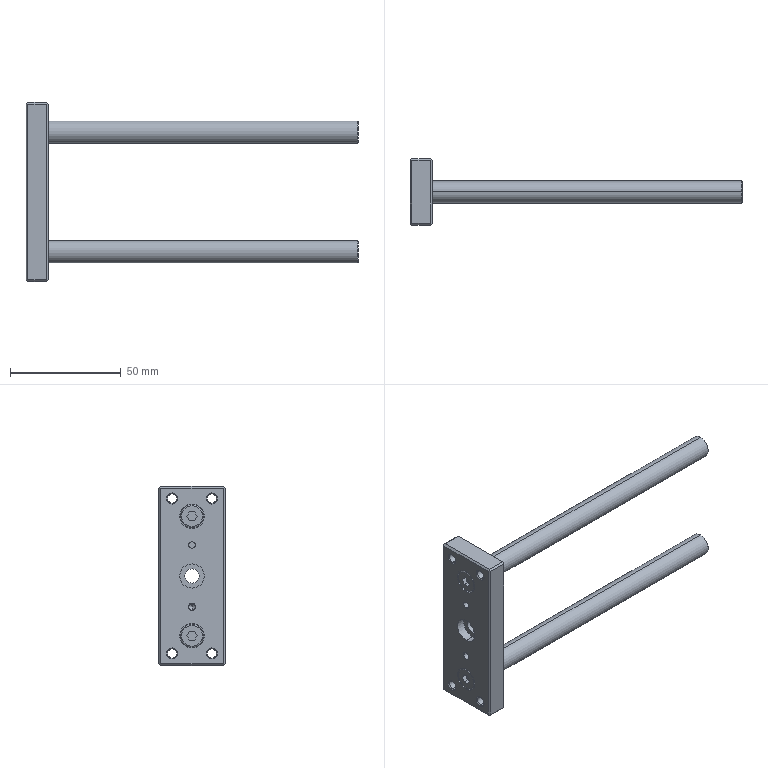Part | STEP file | TC_L_20x70_70fp | 1 solid | 101 faces | box 150 x 30 x 81 mm | volume 44789 mm3 | plane 44 | cylinder 31 | cone 22 | torus 4 | commonest cylinder face diameters 4.134 x8 3 x7 11 x6 10 x4 10.5 x4 6.4 x2